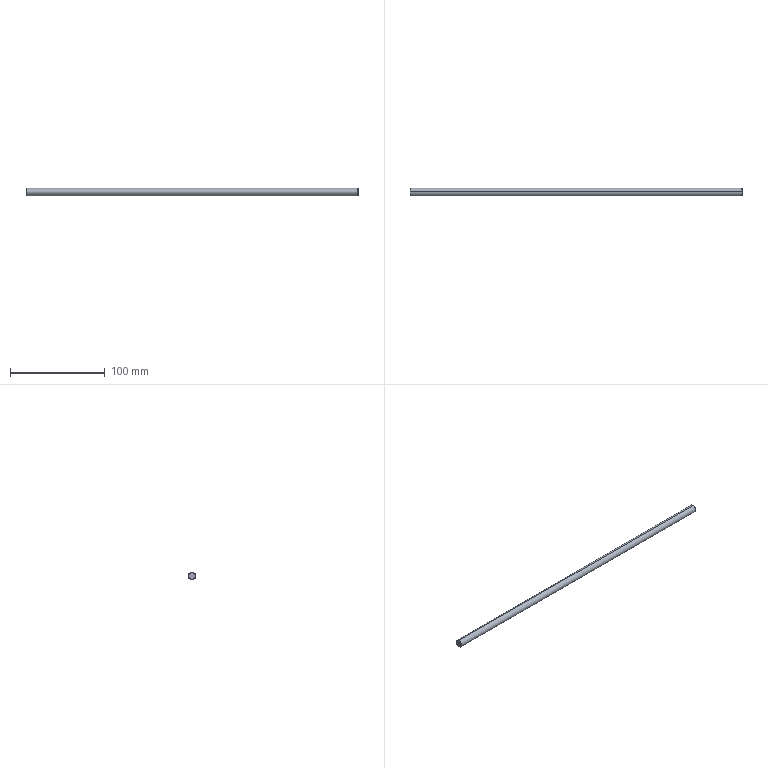Part | SolidWorks | features BaseBody 1 | 1 solid | 8 faces | box 350 x 8 x 8 mm | volume 17587 mm3 | cone 4 | cylinder 2 | plane 2 | commonest cylinder face diameters 8 x2
STEP:
#1=CARTESIAN_POINT('',(0.5,0.,-4.));
#2=VERTEX_POINT('',#1);
#3=CARTESIAN_POINT('',(0.5,0.,4.));
#4=VERTEX_POINT('',#3);
#5=CARTESIAN_POINT('',(0.5,0.,0.));
#6=DIRECTION('',(1.,0.,0.));
#7=DIRECTION('',(0.,0.,-1.));
#8=AXIS2_PLACEMENT_3D('',#5,#6,#7);
#9=CIRCLE('',#8,4.);
#10=EDGE_CURVE('',#2,#4,#9,.T.);
#11=ORIENTED_EDGE('',*,*,#10,.T.);
#12=CARTESIAN_POINT('',(349.5,0.,4.));
#13=VERTEX_POINT('',#12);
#14=CARTESIAN_POINT('',(175.,0.,4.));
#15=DIRECTION('',(1.,0.,0.));
#16=VECTOR('',#15,1000.);
#17=LINE('',#14,#16);
#18=EDGE_CURVE('',#4,#13,#17,.T.);
#19=ORIENTED_EDGE('',*,*,#18,.T.);
#20=CARTESIAN_POINT('',(349.5,0.,-4.));
#21=VERTEX_POINT('',#20);
#22=CARTESIAN_POINT('',(349.5,0.,0.));
#23=DIRECTION('',(-1.,0.,0.));
#24=DIRECTION('',(0.,0.,-1.));
#25=AXIS2_PLACEMENT_3D('',#22,#23,#24);
#26=CIRCLE('',#25,4.);
#27=EDGE_CURVE('',#13,#21,#26,.T.);
#28=ORIENTED_EDGE('',*,*,#27,.T.);
#29=CARTESIAN_POINT('',(175.,0.,-4.));
#30=DIRECTION('',(1.,0.,0.));
#31=VECTOR('',#30,1000.);
#32=LINE('',#29,#31);
#33=EDGE_CURVE('',#2,#21,#32,.T.);
#34=ORIENTED_EDGE('',*,*,#33,.F.);
#35=EDGE_LOOP('',(#11,#19,#28,#34));
#36=FACE_OUTER_BOUND('',#35,.T.);
#37=CARTESIAN_POINT('',(175.,0.,0.));
#38=DIRECTION('',(1.,0.,0.));
#39=DIRECTION('',(0.,0.,-1.));
#40=AXIS2_PLACEMENT_3D('',#37,#38,#39);
#41=CYLINDRICAL_SURFACE('',#40,4.);
#42=ADVANCED_FACE('',(#36),#41,.T.);
#43=CARTESIAN_POINT('',(0.,0.,-3.5));
#44=VERTEX_POINT('',#43);
#45=CARTESIAN_POINT('',(0.,0.,3.5));
#46=VERTEX_POINT('',#45);
#47=CARTESIAN_POINT('',(0.,0.,0.));
#48=DIRECTION('',(1.,0.,0.));
#49=DIRECTION('',(0.,0.,-1.));
#50=AXIS2_PLACEMENT_3D('',#47,#48,#49);
#51=CIRCLE('',#50,3.5);
#52=EDGE_CURVE('',#44,#46,#51,.T.);
#53=ORIENTED_EDGE('',*,*,#52,.T.);
#54=CARTESIAN_POINT('',(0.5,0.,4.));
#55=DIRECTION('',(0.7071,0.,0.7071));
#56=VECTOR('',#55,1000.);
#57=LINE('',#54,#56);
#58=EDGE_CURVE('',#46,#4,#57,.T.);
#59=ORIENTED_EDGE('',*,*,#58,.T.);
#60=ORIENTED_EDGE('',*,*,#10,.F.);
#61=CARTESIAN_POINT('',(0.5,0.,-4.));
#62=DIRECTION('',(0.7071,0.,-0.7071));
#63=VECTOR('',#62,1000.);
#64=LINE('',#61,#63);
#65=EDGE_CURVE('',#44,#2,#64,.T.);
#66=ORIENTED_EDGE('',*,*,#65,.F.);
#67=EDGE_LOOP('',(#53,#59,#60,#66));
#68=FACE_OUTER_BOUND('',#67,.T.);
#69=CARTESIAN_POINT('',(0.5,0.,0.));
#70=DIRECTION('',(1.,0.,0.));
#71=DIRECTION('',(0.,0.,-1.));
#72=AXIS2_PLACEMENT_3D('',#69,#70,#71);
#73=CONICAL_SURFACE('',#72,4.,0.7854);
#74=ADVANCED_FACE('',(#68),#73,.T.);
#75=CARTESIAN_POINT('',(350.,0.,3.5));
#76=VERTEX_POINT('',#75);
#77=CARTESIAN_POINT('',(350.,0.,-3.5));
#78=VERTEX_POINT('',#77);
#79=CARTESIAN_POINT('',(350.,0.,0.));
#80=DIRECTION('',(-1.,0.,0.));
#81=DIRECTION('',(0.,0.,1.));
#82=AXIS2_PLACEMENT_3D('',#79,#80,#81);
#83=CIRCLE('',#82,3.5);
#84=EDGE_CURVE('',#76,#78,#83,.T.);
#85=ORIENTED_EDGE('',*,*,#84,.T.);
#86=CARTESIAN_POINT('',(349.5,0.,-4.));
#87=DIRECTION('',(-0.7071,0.,-0.7071));
#88=VECTOR('',#87,1000.);
#89=LINE('',#86,#88);
#90=EDGE_CURVE('',#78,#21,#89,.T.);
#91=ORIENTED_EDGE('',*,*,#90,.T.);
#92=ORIENTED_EDGE('',*,*,#27,.F.);
#93=CARTESIAN_POINT('',(349.5,0.,4.));
#94=DIRECTION('',(-0.7071,0.,0.7071));
#95=VECTOR('',#94,1000.);
#96=LINE('',#93,#95);
#97=EDGE_CURVE('',#76,#13,#96,.T.);
#98=ORIENTED_EDGE('',*,*,#97,.F.);
#99=EDGE_LOOP('',(#85,#91,#92,#98));
#100=FACE_OUTER_BOUND('',#99,.T.);
#101=CARTESIAN_POINT('',(349.5,0.,0.));
#102=DIRECTION('',(-1.,0.,0.));
#103=DIRECTION('',(0.,0.,1.));
#104=AXIS2_PLACEMENT_3D('',#101,#102,#103);
#105=CONICAL_SURFACE('',#104,4.,0.7854);
#106=ADVANCED_FACE('',(#100),#105,.T.);
#107=ORIENTED_EDGE('',*,*,#18,.F.);
#108=CARTESIAN_POINT('',(0.5,0.,0.));
#109=DIRECTION('',(1.,0.,0.));
#110=DIRECTION('',(0.,0.,-1.));
#111=AXIS2_PLACEMENT_3D('',#108,#109,#110);
#112=CIRCLE('',#111,4.);
#113=EDGE_CURVE('',#4,#2,#112,.T.);
#114=ORIENTED_EDGE('',*,*,#113,.T.);
#115=ORIENTED_EDGE('',*,*,#33,.T.);
#116=CARTESIAN_POINT('',(349.5,0.,0.));
#117=DIRECTION('',(-1.,0.,0.));
#118=DIRECTION('',(0.,0.,-1.));
#119=AXIS2_PLACEMENT_3D('',#116,#117,#118);
#120=CIRCLE('',#119,4.);
#121=EDGE_CURVE('',#21,#13,#120,.T.);
#122=ORIENTED_EDGE('',*,*,#121,.T.);
#123=EDGE_LOOP('',(#107,#114,#115,#122));
#124=FACE_OUTER_BOUND('',#123,.T.);
#125=CARTESIAN_POINT('',(175.,0.,0.));
#126=DIRECTION('',(1.,0.,0.));
#127=DIRECTION('',(0.,0.,-1.));
#128=AXIS2_PLACEMENT_3D('',#125,#126,#127);
#129=CYLINDRICAL_SURFACE('',#128,4.);
#130=ADVANCED_FACE('',(#124),#129,.T.);
#131=ORIENTED_EDGE('',*,*,#58,.F.);
#132=CARTESIAN_POINT('',(0.,0.,0.));
#133=DIRECTION('',(1.,0.,0.));
#134=DIRECTION('',(0.,0.,-1.));
#135=AXIS2_PLACEMENT_3D('',#132,#133,#134);
#136=CIRCLE('',#135,3.5);
#137=EDGE_CURVE('',#46,#44,#136,.T.);
#138=ORIENTED_EDGE('',*,*,#137,.T.);
#139=ORIENTED_EDGE('',*,*,#65,.T.);
#140=ORIENTED_EDGE('',*,*,#113,.F.);
#141=EDGE_LOOP('',(#131,#138,#139,#140));
#142=FACE_OUTER_BOUND('',#141,.T.);
#143=CARTESIAN_POINT('',(0.5,0.,0.));
#144=DIRECTION('',(1.,0.,0.));
#145=DIRECTION('',(0.,0.,-1.));
#146=AXIS2_PLACEMENT_3D('',#143,#144,#145);
#147=CONICAL_SURFACE('',#146,4.,0.7854);
#148=ADVANCED_FACE('',(#142),#147,.T.);
#149=ORIENTED_EDGE('',*,*,#90,.F.);
#150=CARTESIAN_POINT('',(350.,0.,0.));
#151=DIRECTION('',(-1.,0.,0.));
#152=DIRECTION('',(0.,0.,1.));
#153=AXIS2_PLACEMENT_3D('',#150,#151,#152);
#154=CIRCLE('',#153,3.5);
#155=EDGE_CURVE('',#78,#76,#154,.T.);
#156=ORIENTED_EDGE('',*,*,#155,.T.);
#157=ORIENTED_EDGE('',*,*,#97,.T.);
#158=ORIENTED_EDGE('',*,*,#121,.F.);
#159=EDGE_LOOP('',(#149,#156,#157,#158));
#160=FACE_OUTER_BOUND('',#159,.T.);
#161=CARTESIAN_POINT('',(349.5,0.,0.));
#162=DIRECTION('',(-1.,0.,0.));
#163=DIRECTION('',(0.,0.,1.));
#164=AXIS2_PLACEMENT_3D('',#161,#162,#163);
#165=CONICAL_SURFACE('',#164,4.,0.7854);
#166=ADVANCED_FACE('',(#160),#165,.T.);
#167=ORIENTED_EDGE('',*,*,#52,.F.);
#168=ORIENTED_EDGE('',*,*,#137,.F.);
#169=EDGE_LOOP('',(#167,#168));
#170=FACE_OUTER_BOUND('',#169,.T.);
#171=CARTESIAN_POINT('',(0.,1.75,0.));
#172=DIRECTION('',(-1.,0.,0.));
#173=DIRECTION('',(0.,0.,1.));
#174=AXIS2_PLACEMENT_3D('',#171,#172,#173);
#175=PLANE('',#174);
#176=ADVANCED_FACE('',(#170),#175,.T.);
#177=ORIENTED_EDGE('',*,*,#84,.F.);
#178=ORIENTED_EDGE('',*,*,#155,.F.);
#179=EDGE_LOOP('',(#177,#178));
#180=FACE_OUTER_BOUND('',#179,.T.);
#181=CARTESIAN_POINT('',(350.,1.75,0.));
#182=DIRECTION('',(1.,0.,0.));
#183=DIRECTION('',(0.,0.,-1.));
#184=AXIS2_PLACEMENT_3D('',#181,#182,#183);
#185=PLANE('',#184);
#186=ADVANCED_FACE('',(#180),#185,.T.);
#187=CLOSED_SHELL('',(#42,#74,#106,#130,#148,#166,#176,#186));
#188=MANIFOLD_SOLID_BREP('',#187);
#189=CARTESIAN_POINT('',(0.,0.,0.));
#190=DIRECTION('',(0.,0.,1.));
#191=DIRECTION('',(1.,0.,0.));
#192=AXIS2_PLACEMENT_3D('',#189,#190,#191);
#193=(LENGTH_UNIT()NAMED_UNIT(*)SI_UNIT(.MILLI.,.METRE.));
#194=UNCERTAINTY_MEASURE_WITH_UNIT(LENGTH_MEASURE(0.00001),#193,'','');
#195=(NAMED_UNIT(*)PLANE_ANGLE_UNIT()SI_UNIT($,.RADIAN.));
#196=(NAMED_UNIT(*)SI_UNIT($,.STERADIAN.)SOLID_ANGLE_UNIT());
#197=(GEOMETRIC_REPRESENTATION_CONTEXT(3)GLOBAL_UNCERTAINTY_ASSIGNED_CONTEXT((#194))GLOBAL_UNIT_ASSIGNED_CONTEXT((#193,#195,#196))REPRESENTATION_CONTEXT('',''));
#198=ADVANCED_BREP_SHAPE_REPRESENTATION('',(#188,#192),#197);